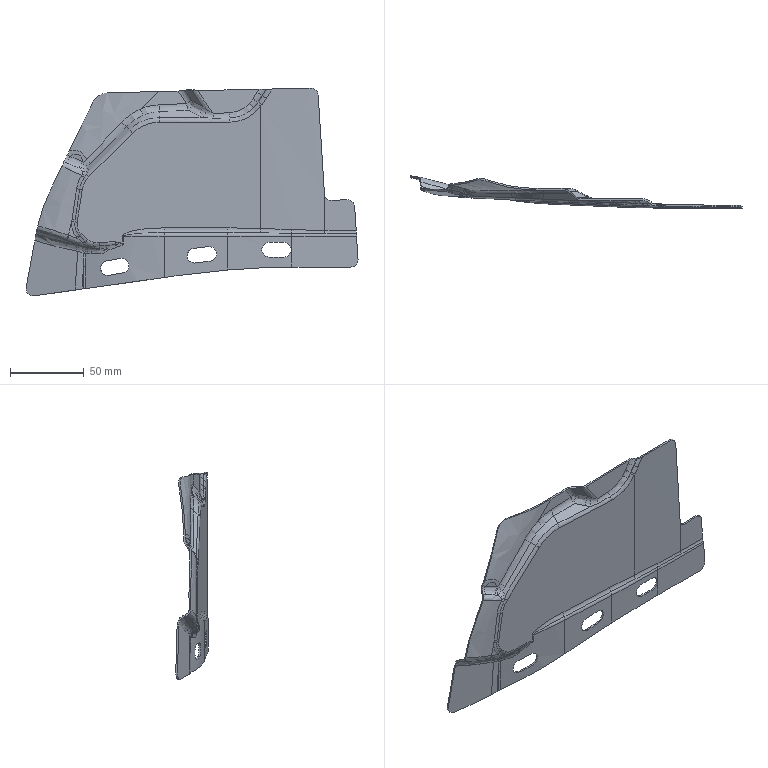Part | STEP file | FNA5401732 | 1 solid | 296 faces | box 225.882 x 22.076 x 141.359 mm | volume 28892 mm3 | spline 240 | plane 25 | cylinder 18 | other 5 | sphere 4 | torus 4 | commonest cylinder face diameters 11.4 x4 13.8 x4 6.2 x2 8.6 x2 1996 x2 1999 x2